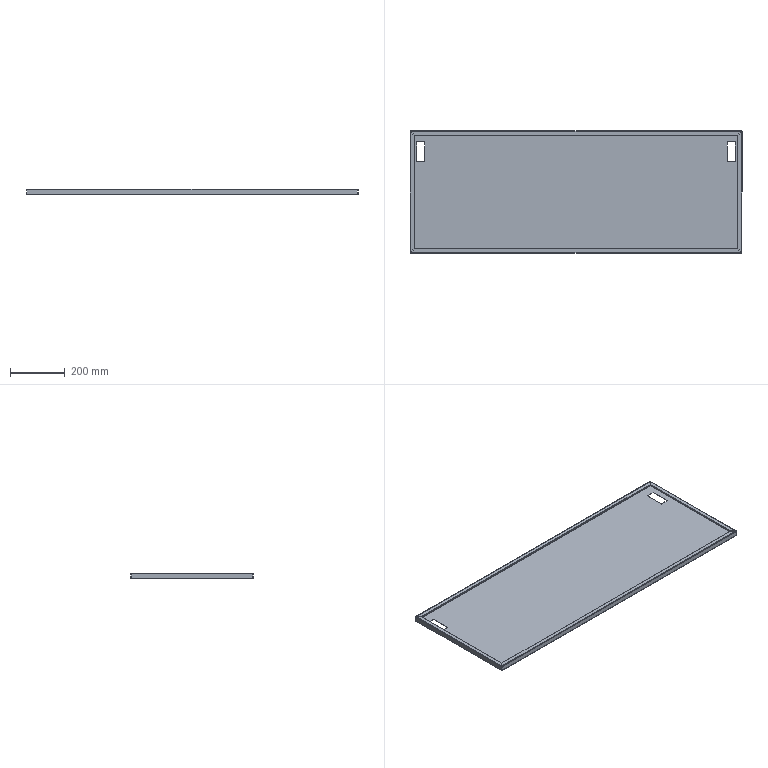Part | SolidWorks | features EdgeFlange 2, FlatPattern 1, SMBaseFlange 1, SheetMetal 1 | 1 solid | 78 faces | box 1218 x 448 x 20 mm | volume 774773 mm3 | plane 46 | spline 16 | cylinder 16 | commonest cylinder face diameters 0.9 x8 3.3 x8